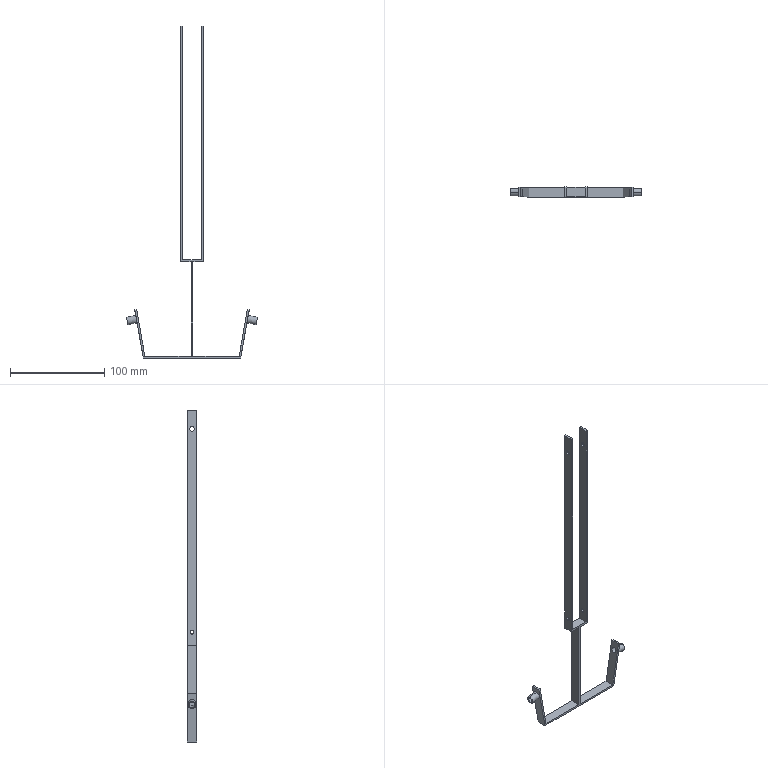Part | SolidWorks | features ICE 6, Extrusion 1, MirrorPattern 1 | 1 solid | 40 faces | box 138.916 x 10 x 352 mm | volume 16665 mm3 | plane 24 | cylinder 16 | commonest cylinder face diameters 4 x4 5 x4 6 x4 8 x4
STEP:
#1=CARTESIAN_POINT('',(12.,5.,10.339));
#2=VERTEX_POINT('',#1);
#3=CARTESIAN_POINT('',(12.,5.,14.339));
#4=VERTEX_POINT('',#3);
#5=CARTESIAN_POINT('',(12.,5.,12.339));
#6=DIRECTION('',(-1.,0.,0.));
#7=DIRECTION('',(0.,0.,1.));
#8=AXIS2_PLACEMENT_3D('',#5,#6,#7);
#9=CIRCLE('',#8,2.);
#10=EDGE_CURVE('',#2,#4,#9,.T.);
#11=ORIENTED_EDGE('',*,*,#10,.F.);
#12=CARTESIAN_POINT('',(10.,5.,10.339));
#13=VERTEX_POINT('',#12);
#14=CARTESIAN_POINT('',(33.,5.,10.339));
#15=DIRECTION('',(-1.,0.,0.));
#16=VECTOR('',#15,1000.);
#17=LINE('',#14,#16);
#18=EDGE_CURVE('',#2,#13,#17,.T.);
#19=ORIENTED_EDGE('',*,*,#18,.T.);
#20=CARTESIAN_POINT('',(10.,5.,14.339));
#21=VERTEX_POINT('',#20);
#22=CARTESIAN_POINT('',(10.,5.,12.339));
#23=DIRECTION('',(1.,0.,0.));
#24=DIRECTION('',(0.,0.,-1.));
#25=AXIS2_PLACEMENT_3D('',#22,#23,#24);
#26=CIRCLE('',#25,2.);
#27=EDGE_CURVE('',#21,#13,#26,.T.);
#28=ORIENTED_EDGE('',*,*,#27,.F.);
#29=CARTESIAN_POINT('',(33.,5.,14.339));
#30=DIRECTION('',(-1.,0.,0.));
#31=VECTOR('',#30,1000.);
#32=LINE('',#29,#31);
#33=EDGE_CURVE('',#4,#21,#32,.T.);
#34=ORIENTED_EDGE('',*,*,#33,.F.);
#35=EDGE_LOOP('',(#11,#19,#28,#34));
#36=FACE_OUTER_BOUND('',#35,.T.);
#37=CARTESIAN_POINT('',(33.,5.,12.339));
#38=DIRECTION('',(-1.,0.,0.));
#39=DIRECTION('',(0.,0.,1.));
#40=AXIS2_PLACEMENT_3D('',#37,#38,#39);
#41=CYLINDRICAL_SURFACE('',#40,2.);
#42=ADVANCED_FACE('',(#36),#41,.F.);
#43=CARTESIAN_POINT('',(-10.,5.,10.339));
#44=VERTEX_POINT('',#43);
#45=CARTESIAN_POINT('',(-10.,5.,14.339));
#46=VERTEX_POINT('',#45);
#47=CARTESIAN_POINT('',(-10.,5.,12.339));
#48=DIRECTION('',(-1.,0.,0.));
#49=DIRECTION('',(0.,0.,1.));
#50=AXIS2_PLACEMENT_3D('',#47,#48,#49);
#51=CIRCLE('',#50,2.);
#52=EDGE_CURVE('',#44,#46,#51,.T.);
#53=ORIENTED_EDGE('',*,*,#52,.F.);
#54=CARTESIAN_POINT('',(-12.,5.,10.339));
#55=VERTEX_POINT('',#54);
#56=CARTESIAN_POINT('',(33.,5.,10.339));
#57=DIRECTION('',(-1.,0.,0.));
#58=VECTOR('',#57,1000.);
#59=LINE('',#56,#58);
#60=EDGE_CURVE('',#44,#55,#59,.T.);
#61=ORIENTED_EDGE('',*,*,#60,.T.);
#62=CARTESIAN_POINT('',(-12.,5.,14.339));
#63=VERTEX_POINT('',#62);
#64=CARTESIAN_POINT('',(-12.,5.,12.339));
#65=DIRECTION('',(-1.,0.,0.));
#66=DIRECTION('',(0.,0.,1.));
#67=AXIS2_PLACEMENT_3D('',#64,#65,#66);
#68=CIRCLE('',#67,2.);
#69=EDGE_CURVE('',#55,#63,#68,.T.);
#70=ORIENTED_EDGE('',*,*,#69,.T.);
#71=CARTESIAN_POINT('',(33.,5.,14.339));
#72=DIRECTION('',(-1.,0.,0.));
#73=VECTOR('',#72,1000.);
#74=LINE('',#71,#73);
#75=EDGE_CURVE('',#46,#63,#74,.T.);
#76=ORIENTED_EDGE('',*,*,#75,.F.);
#77=EDGE_LOOP('',(#53,#61,#70,#76));
#78=FACE_OUTER_BOUND('',#77,.T.);
#79=CARTESIAN_POINT('',(33.,5.,12.339));
#80=DIRECTION('',(-1.,0.,0.));
#81=DIRECTION('',(0.,0.,1.));
#82=AXIS2_PLACEMENT_3D('',#79,#80,#81);
#83=CYLINDRICAL_SURFACE('',#82,2.);
#84=ADVANCED_FACE('',(#78),#83,.F.);
#85=CARTESIAN_POINT('',(12.,5.,225.5));
#86=VERTEX_POINT('',#85);
#87=CARTESIAN_POINT('',(12.,5.,230.5));
#88=VERTEX_POINT('',#87);
#89=CARTESIAN_POINT('',(12.,5.,228.));
#90=DIRECTION('',(-1.,0.,0.));
#91=DIRECTION('',(0.,0.,1.));
#92=AXIS2_PLACEMENT_3D('',#89,#90,#91);
#93=CIRCLE('',#92,2.5);
#94=EDGE_CURVE('',#86,#88,#93,.T.);
#95=ORIENTED_EDGE('',*,*,#94,.F.);
#96=CARTESIAN_POINT('',(10.,5.,225.5));
#97=VERTEX_POINT('',#96);
#98=CARTESIAN_POINT('',(262.,5.,225.5));
#99=DIRECTION('',(-1.,0.,0.));
#100=VECTOR('',#99,1000.);
#101=LINE('',#98,#100);
#102=EDGE_CURVE('',#86,#97,#101,.T.);
#103=ORIENTED_EDGE('',*,*,#102,.T.);
#104=CARTESIAN_POINT('',(10.,5.,230.5));
#105=VERTEX_POINT('',#104);
#106=CARTESIAN_POINT('',(10.,5.,228.));
#107=DIRECTION('',(1.,0.,0.));
#108=DIRECTION('',(0.,0.,-1.));
#109=AXIS2_PLACEMENT_3D('',#106,#107,#108);
#110=CIRCLE('',#109,2.5);
#111=EDGE_CURVE('',#105,#97,#110,.T.);
#112=ORIENTED_EDGE('',*,*,#111,.F.);
#113=CARTESIAN_POINT('',(262.,5.,230.5));
#114=DIRECTION('',(-1.,0.,0.));
#115=VECTOR('',#114,1000.);
#116=LINE('',#113,#115);
#117=EDGE_CURVE('',#88,#105,#116,.T.);
#118=ORIENTED_EDGE('',*,*,#117,.F.);
#119=EDGE_LOOP('',(#95,#103,#112,#118));
#120=FACE_OUTER_BOUND('',#119,.T.);
#121=CARTESIAN_POINT('',(262.,5.,228.));
#122=DIRECTION('',(-1.,0.,0.));
#123=DIRECTION('',(0.,0.,1.));
#124=AXIS2_PLACEMENT_3D('',#121,#122,#123);
#125=CYLINDRICAL_SURFACE('',#124,2.5);
#126=ADVANCED_FACE('',(#120),#125,.F.);
#127=CARTESIAN_POINT('',(-10.,5.,225.5));
#128=VERTEX_POINT('',#127);
#129=CARTESIAN_POINT('',(-10.,5.,230.5));
#130=VERTEX_POINT('',#129);
#131=CARTESIAN_POINT('',(-10.,5.,228.));
#132=DIRECTION('',(-1.,0.,0.));
#133=DIRECTION('',(0.,0.,1.));
#134=AXIS2_PLACEMENT_3D('',#131,#132,#133);
#135=CIRCLE('',#134,2.5);
#136=EDGE_CURVE('',#128,#130,#135,.T.);
#137=ORIENTED_EDGE('',*,*,#136,.F.);
#138=CARTESIAN_POINT('',(-12.,5.,225.5));
#139=VERTEX_POINT('',#138);
#140=CARTESIAN_POINT('',(262.,5.,225.5));
#141=DIRECTION('',(-1.,0.,0.));
#142=VECTOR('',#141,1000.);
#143=LINE('',#140,#142);
#144=EDGE_CURVE('',#128,#139,#143,.T.);
#145=ORIENTED_EDGE('',*,*,#144,.T.);
#146=CARTESIAN_POINT('',(-12.,5.,230.5));
#147=VERTEX_POINT('',#146);
#148=CARTESIAN_POINT('',(-12.,5.,228.));
#149=DIRECTION('',(-1.,0.,0.));
#150=DIRECTION('',(0.,0.,1.));
#151=AXIS2_PLACEMENT_3D('',#148,#149,#150);
#152=CIRCLE('',#151,2.5);
#153=EDGE_CURVE('',#139,#147,#152,.T.);
#154=ORIENTED_EDGE('',*,*,#153,.T.);
#155=CARTESIAN_POINT('',(262.,5.,230.5));
#156=DIRECTION('',(-1.,0.,0.));
#157=VECTOR('',#156,1000.);
#158=LINE('',#155,#157);
#159=EDGE_CURVE('',#130,#147,#158,.T.);
#160=ORIENTED_EDGE('',*,*,#159,.F.);
#161=EDGE_LOOP('',(#137,#145,#154,#160));
#162=FACE_OUTER_BOUND('',#161,.T.);
#163=CARTESIAN_POINT('',(262.,5.,228.));
#164=DIRECTION('',(-1.,0.,0.));
#165=DIRECTION('',(0.,0.,1.));
#166=AXIS2_PLACEMENT_3D('',#163,#164,#165);
#167=CYLINDRICAL_SURFACE('',#166,2.5);
#168=ADVANCED_FACE('',(#162),#167,.F.);
#169=CARTESIAN_POINT('',(68.243,5.,-67.646));
#170=VERTEX_POINT('',#169);
#171=CARTESIAN_POINT('',(69.285,5.,-61.737));
#172=VERTEX_POINT('',#171);
#173=CARTESIAN_POINT('',(68.764,5.,-64.691));
#174=DIRECTION('',(-0.9848,0.,0.1736));
#175=DIRECTION('',(0.1736,0.,0.9848));
#176=AXIS2_PLACEMENT_3D('',#173,#174,#175);
#177=CIRCLE('',#176,3.);
#178=EDGE_CURVE('',#170,#172,#177,.T.);
#179=ORIENTED_EDGE('',*,*,#178,.F.);
#180=CARTESIAN_POINT('',(56.425,5.,-65.562));
#181=VERTEX_POINT('',#180);
#182=CARTESIAN_POINT('',(68.243,5.,-67.646));
#183=DIRECTION('',(-0.9848,0.,0.1736));
#184=VECTOR('',#183,1000.);
#185=LINE('',#182,#184);
#186=EDGE_CURVE('',#170,#181,#185,.T.);
#187=ORIENTED_EDGE('',*,*,#186,.T.);
#188=CARTESIAN_POINT('',(57.467,5.,-59.653));
#189=VERTEX_POINT('',#188);
#190=CARTESIAN_POINT('',(56.946,5.,-62.608));
#191=DIRECTION('',(-0.9848,0.,0.1736));
#192=DIRECTION('',(-0.1736,0.,-0.9848));
#193=AXIS2_PLACEMENT_3D('',#190,#191,#192);
#194=CIRCLE('',#193,3.);
#195=EDGE_CURVE('',#181,#189,#194,.T.);
#196=ORIENTED_EDGE('',*,*,#195,.T.);
#197=CARTESIAN_POINT('',(69.285,5.,-61.737));
#198=DIRECTION('',(-0.9848,0.,0.1736));
#199=VECTOR('',#198,1000.);
#200=LINE('',#197,#199);
#201=EDGE_CURVE('',#172,#189,#200,.T.);
#202=ORIENTED_EDGE('',*,*,#201,.F.);
#203=EDGE_LOOP('',(#179,#187,#196,#202));
#204=FACE_OUTER_BOUND('',#203,.T.);
#205=CARTESIAN_POINT('',(68.764,5.,-64.691));
#206=DIRECTION('',(-0.9848,0.,0.1736));
#207=DIRECTION('',(0.1736,0.,0.9848));
#208=AXIS2_PLACEMENT_3D('',#205,#206,#207);
#209=CYLINDRICAL_SURFACE('',#208,3.);
#210=ADVANCED_FACE('',(#204),#209,.F.);
#211=CARTESIAN_POINT('',(69.458,5.,-60.752));
#212=VERTEX_POINT('',#211);
#213=CARTESIAN_POINT('',(68.069,5.,-68.631));
#214=VERTEX_POINT('',#213);
#215=CARTESIAN_POINT('',(68.764,5.,-64.691));
#216=DIRECTION('',(-0.9848,0.,0.1736));
#217=DIRECTION('',(0.1736,0.,0.9848));
#218=AXIS2_PLACEMENT_3D('',#215,#216,#217);
#219=CIRCLE('',#218,4.);
#220=EDGE_CURVE('',#212,#214,#219,.T.);
#221=ORIENTED_EDGE('',*,*,#220,.T.);
#222=CARTESIAN_POINT('',(58.221,5.,-66.894));
#223=VERTEX_POINT('',#222);
#224=CARTESIAN_POINT('',(68.069,5.,-68.631));
#225=DIRECTION('',(-0.9848,0.,0.1736));
#226=VECTOR('',#225,1000.);
#227=LINE('',#224,#226);
#228=EDGE_CURVE('',#214,#223,#227,.T.);
#229=ORIENTED_EDGE('',*,*,#228,.T.);
#230=CARTESIAN_POINT('',(59.61,5.,-59.016));
#231=VERTEX_POINT('',#230);
#232=CARTESIAN_POINT('',(58.916,5.,-62.955));
#233=DIRECTION('',(-0.9848,0.,0.1736));
#234=DIRECTION('',(0.1736,0.,0.9848));
#235=AXIS2_PLACEMENT_3D('',#232,#233,#234);
#236=CIRCLE('',#235,4.);
#237=EDGE_CURVE('',#231,#223,#236,.T.);
#238=ORIENTED_EDGE('',*,*,#237,.F.);
#239=CARTESIAN_POINT('',(69.458,5.,-60.752));
#240=DIRECTION('',(-0.9848,0.,0.1736));
#241=VECTOR('',#240,1000.);
#242=LINE('',#239,#241);
#243=EDGE_CURVE('',#212,#231,#242,.T.);
#244=ORIENTED_EDGE('',*,*,#243,.F.);
#245=EDGE_LOOP('',(#221,#229,#238,#244));
#246=FACE_OUTER_BOUND('',#245,.T.);
#247=CARTESIAN_POINT('',(68.764,5.,-64.691));
#248=DIRECTION('',(-0.9848,0.,0.1736));
#249=DIRECTION('',(0.1736,0.,0.9848));
#250=AXIS2_PLACEMENT_3D('',#247,#248,#249);
#251=CYLINDRICAL_SURFACE('',#250,4.);
#252=ADVANCED_FACE('',(#246),#251,.T.);
#253=CARTESIAN_POINT('',(-68.243,5.,-67.646));
#254=VERTEX_POINT('',#253);
#255=CARTESIAN_POINT('',(-69.285,5.,-61.737));
#256=VERTEX_POINT('',#255);
#257=CARTESIAN_POINT('',(-68.764,5.,-64.691));
#258=DIRECTION('',(-0.9848,0.,-0.1736));
#259=DIRECTION('',(-0.1736,0.,0.9848));
#260=AXIS2_PLACEMENT_3D('',#257,#258,#259);
#261=CIRCLE('',#260,3.);
#262=EDGE_CURVE('',#254,#256,#261,.T.);
#263=ORIENTED_EDGE('',*,*,#262,.T.);
#264=CARTESIAN_POINT('',(-57.467,5.,-59.653));
#265=VERTEX_POINT('',#264);
#266=CARTESIAN_POINT('',(-69.285,5.,-61.737));
#267=DIRECTION('',(0.9848,0.,0.1736));
#268=VECTOR('',#267,1000.);
#269=LINE('',#266,#268);
#270=EDGE_CURVE('',#256,#265,#269,.T.);
#271=ORIENTED_EDGE('',*,*,#270,.T.);
#272=CARTESIAN_POINT('',(-56.425,5.,-65.562));
#273=VERTEX_POINT('',#272);
#274=CARTESIAN_POINT('',(-56.946,5.,-62.608));
#275=DIRECTION('',(-0.9848,0.,-0.1736));
#276=DIRECTION('',(-0.1736,0.,0.9848));
#277=AXIS2_PLACEMENT_3D('',#274,#275,#276);
#278=CIRCLE('',#277,3.);
#279=EDGE_CURVE('',#273,#265,#278,.T.);
#280=ORIENTED_EDGE('',*,*,#279,.F.);
#281=CARTESIAN_POINT('',(-68.243,5.,-67.646));
#282=DIRECTION('',(0.9848,0.,0.1736));
#283=VECTOR('',#282,1000.);
#284=LINE('',#281,#283);
#285=EDGE_CURVE('',#254,#273,#284,.T.);
#286=ORIENTED_EDGE('',*,*,#285,.F.);
#287=EDGE_LOOP('',(#263,#271,#280,#286));
#288=FACE_OUTER_BOUND('',#287,.T.);
#289=CARTESIAN_POINT('',(-68.764,5.,-64.691));
#290=DIRECTION('',(0.9848,0.,0.1736));
#291=DIRECTION('',(0.1736,0.,-0.9848));
#292=AXIS2_PLACEMENT_3D('',#289,#290,#291);
#293=CYLINDRICAL_SURFACE('',#292,3.);
#294=ADVANCED_FACE('',(#288),#293,.F.);
#295=CARTESIAN_POINT('',(-69.458,5.,-60.752));
#296=VERTEX_POINT('',#295);
#297=CARTESIAN_POINT('',(-68.069,5.,-68.631));
#298=VERTEX_POINT('',#297);
#299=CARTESIAN_POINT('',(-68.764,5.,-64.691));
#300=DIRECTION('',(-0.9848,0.,-0.1736));
#301=DIRECTION('',(-0.1736,0.,0.9848));
#302=AXIS2_PLACEMENT_3D('',#299,#300,#301);
#303=CIRCLE('',#302,4.);
#304=EDGE_CURVE('',#296,#298,#303,.T.);
#305=ORIENTED_EDGE('',*,*,#304,.F.);
#306=CARTESIAN_POINT('',(-59.61,5.,-59.016));
#307=VERTEX_POINT('',#306);
#308=CARTESIAN_POINT('',(-69.458,5.,-60.752));
#309=DIRECTION('',(0.9848,0.,0.1736));
#310=VECTOR('',#309,1000.);
#311=LINE('',#308,#310);
#312=EDGE_CURVE('',#296,#307,#311,.T.);
#313=ORIENTED_EDGE('',*,*,#312,.T.);
#314=CARTESIAN_POINT('',(-58.221,5.,-66.894));
#315=VERTEX_POINT('',#314);
#316=CARTESIAN_POINT('',(-58.916,5.,-62.955));
#317=DIRECTION('',(-0.9848,0.,-0.1736));
#318=DIRECTION('',(0.1736,0.,-0.9848));
#319=AXIS2_PLACEMENT_3D('',#316,#317,#318);
#320=CIRCLE('',#319,4.);
#321=EDGE_CURVE('',#307,#315,#320,.T.);
#322=ORIENTED_EDGE('',*,*,#321,.T.);
#323=CARTESIAN_POINT('',(-68.069,5.,-68.631));
#324=DIRECTION('',(0.9848,0.,0.1736));
#325=VECTOR('',#324,1000.);
#326=LINE('',#323,#325);
#327=EDGE_CURVE('',#298,#315,#326,.T.);
#328=ORIENTED_EDGE('',*,*,#327,.F.);
#329=EDGE_LOOP('',(#305,#313,#322,#328));
#330=FACE_OUTER_BOUND('',#329,.T.);
#331=CARTESIAN_POINT('',(-68.764,5.,-64.691));
#332=DIRECTION('',(0.9848,0.,0.1736));
#333=DIRECTION('',(0.1736,0.,-0.9848));
#334=AXIS2_PLACEMENT_3D('',#331,#332,#333);
#335=CYLINDRICAL_SURFACE('',#334,4.);
#336=ADVANCED_FACE('',(#330),#335,.T.);
#337=CARTESIAN_POINT('',(1.,10.,-2.));
#338=VERTEX_POINT('',#337);
#339=CARTESIAN_POINT('',(1.,0.,-2.));
#340=VERTEX_POINT('',#339);
#341=CARTESIAN_POINT('',(1.,0.,-2.));
#342=DIRECTION('',(0.,-1.,0.));
#343=VECTOR('',#342,1000.);
#344=LINE('',#341,#343);
#345=EDGE_CURVE('',#338,#340,#344,.T.);
#346=ORIENTED_EDGE('',*,*,#345,.F.);
#347=CARTESIAN_POINT('',(12.,10.,-2.));
#348=VERTEX_POINT('',#347);
#349=CARTESIAN_POINT('',(-12.,10.,-2.));
#350=DIRECTION('',(-1.,0.,0.));
#351=VECTOR('',#350,1000.);
#352=LINE('',#349,#351);
#353=EDGE_CURVE('',#348,#338,#352,.T.);
#354=ORIENTED_EDGE('',*,*,#353,.F.);
#355=CARTESIAN_POINT('',(12.,0.,-2.));
#356=VERTEX_POINT('',#355);
#357=CARTESIAN_POINT('',(12.,10.,-2.));
#358=DIRECTION('',(0.,-1.,0.));
#359=VECTOR('',#358,1000.);
#360=LINE('',#357,#359);
#361=EDGE_CURVE('',#348,#356,#360,.T.);
#362=ORIENTED_EDGE('',*,*,#361,.T.);
#363=CARTESIAN_POINT('',(-12.,0.,-2.));
#364=DIRECTION('',(-1.,0.,0.));
#365=VECTOR('',#364,1000.);
#366=LINE('',#363,#365);
#367=EDGE_CURVE('',#356,#340,#366,.T.);
#368=ORIENTED_EDGE('',*,*,#367,.T.);
#369=EDGE_LOOP('',(#346,#354,#362,#368));
#370=FACE_OUTER_BOUND('',#369,.T.);
#371=CARTESIAN_POINT('',(-12.,10.,-2.));
#372=DIRECTION('',(0.,0.,1.));
#373=DIRECTION('',(1.,0.,0.));
#374=AXIS2_PLACEMENT_3D('',#371,#372,#373);
#375=PLANE('',#374);
#376=ADVANCED_FACE('',(#370),#375,.F.);
#377=CARTESIAN_POINT('',(-12.,0.,248.));
#378=VERTEX_POINT('',#377);
#379=CARTESIAN_POINT('',(-10.,0.,248.));
#380=VERTEX_POINT('',#379);
#381=CARTESIAN_POINT('',(-12.,0.,248.));
#382=DIRECTION('',(1.,0.,0.));
#383=VECTOR('',#382,1000.);
#384=LINE('',#381,#383);
#385=EDGE_CURVE('',#378,#380,#384,.T.);
#386=ORIENTED_EDGE('',*,*,#385,.T.);
#387=CARTESIAN_POINT('',(-10.,10.,248.));
#388=VERTEX_POINT('',#387);
#389=CARTESIAN_POINT('',(-10.,10.,248.));
#390=DIRECTION('',(0.,-1.,0.));
#391=VECTOR('',#390,1000.);
#392=LINE('',#389,#391);
#393=EDGE_CURVE('',#388,#380,#392,.T.);
#394=ORIENTED_EDGE('',*,*,#393,.F.);
#395=CARTESIAN_POINT('',(-12.,10.,248.));
#396=VERTEX_POINT('',#395);
#397=CARTESIAN_POINT('',(-12.,10.,248.));
#398=DIRECTION('',(1.,0.,0.));
#399=VECTOR('',#398,1000.);
#400=LINE('',#397,#399);
#401=EDGE_CURVE('',#396,#388,#400,.T.);
#402=ORIENTED_EDGE('',*,*,#401,.F.);
#403=CARTESIAN_POINT('',(-12.,10.,248.));
#404=DIRECTION('',(0.,-1.,0.));
#405=VECTOR('',#404,1000.);
#406=LINE('',#403,#405);
#407=EDGE_CURVE('',#396,#378,#406,.T.);
#408=ORIENTED_EDGE('',*,*,#407,.T.);
#409=EDGE_LOOP('',(#386,#394,#402,#408));
#410=FACE_OUTER_BOUND('',#409,.T.);
#411=CARTESIAN_POINT('',(-12.,10.,248.));
#412=DIRECTION('',(0.,0.,-1.));
#413=DIRECTION('',(-1.,0.,0.));
#414=AXIS2_PLACEMENT_3D('',#411,#412,#413);
#415=PLANE('',#414);
#416=ADVANCED_FACE('',(#410),#415,.F.);
#417=CARTESIAN_POINT('',(-10.,5.,12.339));
#418=DIRECTION('',(-1.,0.,0.));
#419=DIRECTION('',(0.,0.,1.));
#420=AXIS2_PLACEMENT_3D('',#417,#418,#419);
#421=CIRCLE('',#420,2.);
#422=EDGE_CURVE('',#46,#44,#421,.T.);
#423=ORIENTED_EDGE('',*,*,#422,.T.);
#424=ORIENTED_EDGE('',*,*,#52,.T.);
#425=EDGE_LOOP('',(#423,#424));
#426=FACE_BOUND('',#425,.T.);
#427=CARTESIAN_POINT('',(-10.,5.,228.));
#428=DIRECTION('',(-1.,0.,0.));
#429=DIRECTION('',(0.,0.,1.));
#430=AXIS2_PLACEMENT_3D('',#427,#428,#429);
#431=CIRCLE('',#430,2.5);
#432=EDGE_CURVE('',#130,#128,#431,.T.);
#433=ORIENTED_EDGE('',*,*,#432,.T.);
#434=ORIENTED_EDGE('',*,*,#136,.T.);
#435=EDGE_LOOP('',(#433,#434));
#436=FACE_BOUND('',#435,.T.);
#437=CARTESIAN_POINT('',(-10.,0.,0.));
#438=VERTEX_POINT('',#437);
#439=CARTESIAN_POINT('',(-10.,0.,248.));
#440=DIRECTION('',(0.,0.,-1.));
#441=VECTOR('',#440,1000.);
#442=LINE('',#439,#441);
#443=EDGE_CURVE('',#380,#438,#442,.T.);
#444=ORIENTED_EDGE('',*,*,#443,.T.);
#445=CARTESIAN_POINT('',(-10.,10.,0.));
#446=VERTEX_POINT('',#445);
#447=CARTESIAN_POINT('',(-10.,10.,0.));
#448=DIRECTION('',(0.,-1.,0.));
#449=VECTOR('',#448,1000.);
#450=LINE('',#447,#449);
#451=EDGE_CURVE('',#446,#438,#450,.T.);
#452=ORIENTED_EDGE('',*,*,#451,.F.);
#453=CARTESIAN_POINT('',(-10.,10.,248.));
#454=DIRECTION('',(0.,0.,-1.));
#455=VECTOR('',#454,1000.);
#456=LINE('',#453,#455);
#457=EDGE_CURVE('',#388,#446,#456,.T.);
#458=ORIENTED_EDGE('',*,*,#457,.F.);
#459=ORIENTED_EDGE('',*,*,#393,.T.);
#460=EDGE_LOOP('',(#444,#452,#458,#459));
#461=FACE_OUTER_BOUND('',#460,.T.);
#462=CARTESIAN_POINT('',(-10.,10.,248.));
#463=DIRECTION('',(-1.,0.,0.));
#464=DIRECTION('',(0.,0.,1.));
#465=AXIS2_PLACEMENT_3D('',#462,#463,#464);
#466=PLANE('',#465);
#467=ADVANCED_FACE('',(#426,#436,#461),#466,.F.);
#468=CARTESIAN_POINT('',(10.,0.,0.));
#469=VERTEX_POINT('',#468);
#470=CARTESIAN_POINT('',(-10.,0.,0.));
#471=DIRECTION('',(1.,0.,0.));
#472=VECTOR('',#471,1000.);
#473=LINE('',#470,#472);
#474=EDGE_CURVE('',#438,#469,#473,.T.);
#475=ORIENTED_EDGE('',*,*,#474,.T.);
#476=CARTESIAN_POINT('',(10.,10.,0.));
#477=VERTEX_POINT('',#476);
#478=CARTESIAN_POINT('',(10.,10.,0.));
#479=DIRECTION('',(0.,-1.,0.));
#480=VECTOR('',#479,1000.);
#481=LINE('',#478,#480);
#482=EDGE_CURVE('',#477,#469,#481,.T.);
#483=ORIENTED_EDGE('',*,*,#482,.F.);
#484=CARTESIAN_POINT('',(-10.,10.,0.));
#485=DIRECTION('',(1.,0.,0.));
#486=VECTOR('',#485,1000.);
#487=LINE('',#484,#486);
#488=EDGE_CURVE('',#446,#477,#487,.T.);
#489=ORIENTED_EDGE('',*,*,#488,.F.);
#490=ORIENTED_EDGE('',*,*,#451,.T.);
#491=EDGE_LOOP('',(#475,#483,#489,#490));
#492=FACE_OUTER_BOUND('',#491,.T.);
#493=CARTESIAN_POINT('',(-10.,10.,0.));
#494=DIRECTION('',(0.,0.,-1.));
#495=DIRECTION('',(-1.,0.,0.));
#496=AXIS2_PLACEMENT_3D('',#493,#494,#495);
#497=PLANE('',#496);
#498=ADVANCED_FACE('',(#492),#497,.F.);
#499=ORIENTED_EDGE('',*,*,#27,.T.);
#500=CARTESIAN_POINT('',(10.,5.,12.339));
#501=DIRECTION('',(1.,0.,0.));
#502=DIRECTION('',(0.,0.,-1.));
#503=AXIS2_PLACEMENT_3D('',#500,#501,#502);
#504=CIRCLE('',#503,2.);
#505=EDGE_CURVE('',#13,#21,#504,.T.);
#506=ORIENTED_EDGE('',*,*,#505,.T.);
#507=EDGE_LOOP('',(#499,#506));
#508=FACE_BOUND('',#507,.T.);
#509=ORIENTED_EDGE('',*,*,#111,.T.);
#510=CARTESIAN_POINT('',(10.,5.,228.));
#511=DIRECTION('',(1.,0.,0.));
#512=DIRECTION('',(0.,0.,-1.));
#513=AXIS2_PLACEMENT_3D('',#510,#511,#512);
#514=CIRCLE('',#513,2.5);
#515=EDGE_CURVE('',#97,#105,#514,.T.);
#516=ORIENTED_EDGE('',*,*,#515,.T.);
#517=EDGE_LOOP('',(#509,#516));
#518=FACE_BOUND('',#517,.T.);
#519=CARTESIAN_POINT('',(10.,0.,248.));
#520=VERTEX_POINT('',#519);
#521=CARTESIAN_POINT('',(10.,0.,0.));
#522=DIRECTION('',(0.,0.,1.));
#523=VECTOR('',#522,1000.);
#524=LINE('',#521,#523);
#525=EDGE_CURVE('',#469,#520,#524,.T.);
#526=ORIENTED_EDGE('',*,*,#525,.T.);
#527=CARTESIAN_POINT('',(10.,10.,248.));
#528=VERTEX_POINT('',#527);
#529=CARTESIAN_POINT('',(10.,10.,248.));
#530=DIRECTION('',(0.,-1.,0.));
#531=VECTOR('',#530,1000.);
#532=LINE('',#529,#531);
#533=EDGE_CURVE('',#528,#520,#532,.T.);
#534=ORIENTED_EDGE('',*,*,#533,.F.);
#535=CARTESIAN_POINT('',(10.,10.,0.));
#536=DIRECTION('',(0.,0.,1.));
#537=VECTOR('',#536,1000.);
#538=LINE('',#535,#537);
#539=EDGE_CURVE('',#477,#528,#538,.T.);
#540=ORIENTED_EDGE('',*,*,#539,.F.);
#541=ORIENTED_EDGE('',*,*,#482,.T.);
#542=EDGE_LOOP('',(#526,#534,#540,#541));
#543=FACE_OUTER_BOUND('',#542,.T.);
#544=CARTESIAN_POINT('',(10.,10.,0.));
#545=DIRECTION('',(1.,0.,0.));
#546=DIRECTION('',(0.,0.,-1.));
#547=AXIS2_PLACEMENT_3D('',#544,#545,#546);
#548=PLANE('',#547);
#549=ADVANCED_FACE('',(#508,#518,#543),#548,.F.);
#550=CARTESIAN_POINT('',(12.,0.,248.));
#551=VERTEX_POINT('',#550);
#552=CARTESIAN_POINT('',(10.,0.,248.));
#553=DIRECTION('',(1.,0.,0.));
#554=VECTOR('',#553,1000.);
#555=LINE('',#552,#554);
#556=EDGE_CURVE('',#520,#551,#555,.T.);
#557=ORIENTED_EDGE('',*,*,#556,.T.);
#558=CARTESIAN_POINT('',(12.,10.,248.));
#559=VERTEX_POINT('',#558);
#560=CARTESIAN_POINT('',(12.,10.,248.));
#561=DIRECTION('',(0.,-1.,0.));
#562=VECTOR('',#561,1000.);
#563=LINE('',#560,#562);
#564=EDGE_CURVE('',#559,#551,#563,.T.);
#565=ORIENTED_EDGE('',*,*,#564,.F.);
#566=CARTESIAN_POINT('',(10.,10.,248.));
#567=DIRECTION('',(1.,0.,0.));
#568=VECTOR('',#567,1000.);
#569=LINE('',#566,#568);
#570=EDGE_CURVE('',#528,#559,#569,.T.);
#571=ORIENTED_EDGE('',*,*,#570,.F.);
#572=ORIENTED_EDGE('',*,*,#533,.T.);
#573=EDGE_LOOP('',(#557,#565,#571,#572));
#574=FACE_OUTER_BOUND('',#573,.T.);
#575=CARTESIAN_POINT('',(10.,10.,248.));
#576=DIRECTION('',(0.,0.,-1.));
#577=DIRECTION('',(-1.,0.,0.));
#578=AXIS2_PLACEMENT_3D('',#575,#576,#577);
#579=PLANE('',#578);
#580=ADVANCED_FACE('',(#574),#579,.F.);
#581=CARTESIAN_POINT('',(12.,5.,12.339));
#582=DIRECTION('',(-1.,0.,0.));
#583=DIRECTION('',(0.,0.,1.));
#584=AXIS2_PLACEMENT_3D('',#581,#582,#583);
#585=CIRCLE('',#584,2.);
#586=EDGE_CURVE('',#4,#2,#585,.T.);
#587=ORIENTED_EDGE('',*,*,#586,.T.);
#588=ORIENTED_EDGE('',*,*,#10,.T.);
#589=EDGE_LOOP('',(#587,#588));
#590=FACE_BOUND('',#589,.T.);
#591=CARTESIAN_POINT('',(12.,5.,228.));
#592=DIRECTION('',(-1.,0.,0.));
#593=DIRECTION('',(0.,0.,1.));
#594=AXIS2_PLACEMENT_3D('',#591,#592,#593);
#595=CIRCLE('',#594,2.5);
#596=EDGE_CURVE('',#88,#86,#595,.T.);
#597=ORIENTED_EDGE('',*,*,#596,.T.);
#598=ORIENTED_EDGE('',*,*,#94,.T.);
#599=EDGE_LOOP('',(#597,#598));
#600=FACE_BOUND('',#599,.T.);
#601=CARTESIAN_POINT('',(12.,0.,-2.));
#602=DIRECTION('',(0.,0.,-1.));
#603=VECTOR('',#602,1000.);
#604=LINE('',#601,#603);
#605=EDGE_CURVE('',#551,#356,#604,.T.);
#606=ORIENTED_EDGE('',*,*,#605,.T.);
#607=ORIENTED_EDGE('',*,*,#361,.F.);
#608=CARTESIAN_POINT('',(12.,10.,-2.));
#609=DIRECTION('',(0.,0.,-1.));
#610=VECTOR('',#609,1000.);
#611=LINE('',#608,#610);
#612=EDGE_CURVE('',#559,#348,#611,.T.);
#613=ORIENTED_EDGE('',*,*,#612,.F.);
#614=ORIENTED_EDGE('',*,*,#564,.T.);
#615=EDGE_LOOP('',(#606,#607,#613,#614));
#616=FACE_OUTER_BOUND('',#615,.T.);
#617=CARTESIAN_POINT('',(12.,10.,-2.));
#618=DIRECTION('',(-1.,0.,0.));
#619=DIRECTION('',(0.,0.,1.));
#620=AXIS2_PLACEMENT_3D('',#617,#618,#619);
#621=PLANE('',#620);
#622=ADVANCED_FACE('',(#590,#600,#616),#621,.F.);
#623=CARTESIAN_POINT('',(-1.,10.,-2.));
#624=VERTEX_POINT('',#623);
#625=CARTESIAN_POINT('',(-12.,10.,-2.));
#626=VERTEX_POINT('',#625);
#627=CARTESIAN_POINT('',(-12.,10.,-2.));
#628=DIRECTION('',(-1.,0.,0.));
#629=VECTOR('',#628,1000.);
#630=LINE('',#627,#629);
#631=EDGE_CURVE('',#624,#626,#630,.T.);
#632=ORIENTED_EDGE('',*,*,#631,.F.);
#633=CARTESIAN_POINT('',(-1.,0.,-2.));
#634=VERTEX_POINT('',#633);
#635=CARTESIAN_POINT('',(-1.,0.,-2.));
#636=DIRECTION('',(0.,-1.,0.));
#637=VECTOR('',#636,1000.);
#638=LINE('',#635,#637);
#639=EDGE_CURVE('',#624,#634,#638,.T.);
#640=ORIENTED_EDGE('',*,*,#639,.T.);
#641=CARTESIAN_POINT('',(-12.,0.,-2.));
#642=VERTEX_POINT('',#641);
#643=CARTESIAN_POINT('',(-12.,0.,-2.));
#644=DIRECTION('',(-1.,0.,0.));
#645=VECTOR('',#644,1000.);
#646=LINE('',#643,#645);
#647=EDGE_CURVE('',#634,#642,#646,.T.);
#648=ORIENTED_EDGE('',*,*,#647,.T.);
#649=CARTESIAN_POINT('',(-12.,10.,-2.));
#650=DIRECTION('',(0.,-1.,0.));
#651=VECTOR('',#650,1000.);
#652=LINE('',#649,#651);
#653=EDGE_CURVE('',#626,#642,#652,.T.);
#654=ORIENTED_EDGE('',*,*,#653,.F.);
#655=EDGE_LOOP('',(#632,#640,#648,#654));
#656=FACE_OUTER_BOUND('',#655,.T.);
#657=CARTESIAN_POINT('',(-12.,10.,-2.));
#658=DIRECTION('',(0.,0.,1.));
#659=DIRECTION('',(1.,0.,0.));
#660=AXIS2_PLACEMENT_3D('',#657,#658,#659);
#661=PLANE('',#660);
#662=ADVANCED_FACE('',(#656),#661,.F.);
#663=CARTESIAN_POINT('',(-12.,5.,12.339));
#664=DIRECTION('',(-1.,0.,0.));
#665=DIRECTION('',(0.,0.,1.));
#666=AXIS2_PLACEMENT_3D('',#663,#664,#665);
#667=CIRCLE('',#666,2.);
#668=EDGE_CURVE('',#63,#55,#667,.T.);
#669=ORIENTED_EDGE('',*,*,#668,.F.);
#670=ORIENTED_EDGE('',*,*,#69,.F.);
#671=EDGE_LOOP('',(#669,#670));
#672=FACE_BOUND('',#671,.T.);
#673=CARTESIAN_POINT('',(-12.,5.,228.));
#674=DIRECTION('',(-1.,0.,0.));
#675=DIRECTION('',(0.,0.,1.));
#676=AXIS2_PLACEMENT_3D('',#673,#674,#675);
#677=CIRCLE('',#676,2.5);
#678=EDGE_CURVE('',#147,#139,#677,.T.);
#679=ORIENTED_EDGE('',*,*,#678,.F.);
#680=ORIENTED_EDGE('',*,*,#153,.F.);
#681=EDGE_LOOP('',(#679,#680));
#682=FACE_BOUND('',#681,.T.);
#683=CARTESIAN_POINT('',(-12.,0.,248.));
#684=DIRECTION('',(0.,0.,1.));
#685=VECTOR('',#684,1000.);
#686=LINE('',#683,#685);
#687=EDGE_CURVE('',#642,#378,#686,.T.);
#688=ORIENTED_EDGE('',*,*,#687,.T.);
#689=ORIENTED_EDGE('',*,*,#407,.F.);
#690=CARTESIAN_POINT('',(-12.,10.,248.));
#691=DIRECTION('',(0.,0.,1.));
#692=VECTOR('',#691,1000.);
#693=LINE('',#690,#692);
#694=EDGE_CURVE('',#626,#396,#693,.T.);
#695=ORIENTED_EDGE('',*,*,#694,.F.);
#696=ORIENTED_EDGE('',*,*,#653,.T.);
#697=EDGE_LOOP('',(#688,#689,#695,#696));
#698=FACE_OUTER_BOUND('',#697,.T.);
#699=CARTESIAN_POINT('',(-12.,10.,248.));
#700=DIRECTION('',(1.,0.,0.));
#701=DIRECTION('',(0.,0.,-1.));
#702=AXIS2_PLACEMENT_3D('',#699,#700,#701);
#703=PLANE('',#702);
#704=ADVANCED_FACE('',(#672,#682,#698),#703,.F.);
#705=ORIENTED_EDGE('',*,*,#401,.T.);
#706=ORIENTED_EDGE('',*,*,#457,.T.);
#707=ORIENTED_EDGE('',*,*,#488,.T.);
#708=ORIENTED_EDGE('',*,*,#539,.T.);
#709=ORIENTED_EDGE('',*,*,#570,.T.);
#710=ORIENTED_EDGE('',*,*,#612,.T.);
#711=ORIENTED_EDGE('',*,*,#353,.T.);
#712=CARTESIAN_POINT('',(1.,10.,-102.));
#713=VERTEX_POINT('',#712);
#714=CARTESIAN_POINT('',(1.,10.,-2.));
#715=DIRECTION('',(0.,0.,1.));
#716=VECTOR('',#715,1000.);
#717=LINE('',#714,#716);
#718=EDGE_CURVE('',#713,#338,#717,.T.);
#719=ORIENTED_EDGE('',*,*,#718,.F.);
#720=CARTESIAN_POINT('',(50.,10.,-102.));
#721=VERTEX_POINT('',#720);
#722=CARTESIAN_POINT('',(-50.,10.,-102.));
#723=DIRECTION('',(1.,0.,0.));
#724=VECTOR('',#723,1000.);
#725=LINE('',#722,#724);
#726=EDGE_CURVE('',#713,#721,#725,.T.);
#727=ORIENTED_EDGE('',*,*,#726,.T.);
#728=CARTESIAN_POINT('',(58.682,10.,-52.76));
#729=VERTEX_POINT('',#728);
#730=CARTESIAN_POINT('',(50.,10.,-102.));
#731=DIRECTION('',(0.1736,0.,0.9848));
#732=VECTOR('',#731,1000.);
#733=LINE('',#730,#732);
#734=EDGE_CURVE('',#721,#729,#733,.T.);
#735=ORIENTED_EDGE('',*,*,#734,.T.);
#736=CARTESIAN_POINT('',(60.652,10.,-53.107));
#737=VERTEX_POINT('',#736);
#738=CARTESIAN_POINT('',(60.652,10.,-53.107));
#739=DIRECTION('',(0.9848,0.,-0.1736));
#740=VECTOR('',#739,1000.);
#741=LINE('',#738,#740);
#742=EDGE_CURVE('',#729,#737,#741,.T.);
#743=ORIENTED_EDGE('',*,*,#742,.T.);
#744=CARTESIAN_POINT('',(51.678,10.,-104.));
#745=VERTEX_POINT('',#744);
#746=CARTESIAN_POINT('',(51.678,10.,-104.));
#747=DIRECTION('',(-0.1736,0.,-0.9848));
#748=VECTOR('',#747,1000.);
#749=LINE('',#746,#748);
#750=EDGE_CURVE('',#737,#745,#749,.T.);
#751=ORIENTED_EDGE('',*,*,#750,.T.);
#752=CARTESIAN_POINT('',(-51.678,10.,-104.));
#753=VERTEX_POINT('',#752);
#754=CARTESIAN_POINT('',(-51.678,10.,-104.));
#755=DIRECTION('',(-1.,0.,0.));
#756=VECTOR('',#755,1000.);
#757=LINE('',#754,#756);
#758=EDGE_CURVE('',#745,#753,#757,.T.);
#759=ORIENTED_EDGE('',*,*,#758,.T.);
#760=CARTESIAN_POINT('',(-60.652,10.,-53.107));
#761=VERTEX_POINT('',#760);
#762=CARTESIAN_POINT('',(-51.678,10.,-104.));
#763=DIRECTION('',(-0.1736,0.,0.9848));
#764=VECTOR('',#763,1000.);
#765=LINE('',#762,#764);
#766=EDGE_CURVE('',#753,#761,#765,.T.);
#767=ORIENTED_EDGE('',*,*,#766,.T.);
#768=CARTESIAN_POINT('',(-58.682,10.,-52.76));
#769=VERTEX_POINT('',#768);
#770=CARTESIAN_POINT('',(-58.682,10.,-52.76));
#771=DIRECTION('',(0.9848,0.,0.1736));
#772=VECTOR('',#771,1000.);
#773=LINE('',#770,#772);
#774=EDGE_CURVE('',#761,#769,#773,.T.);
#775=ORIENTED_EDGE('',*,*,#774,.T.);
#776=CARTESIAN_POINT('',(-50.,10.,-102.));
#777=VERTEX_POINT('',#776);
#778=CARTESIAN_POINT('',(-50.,10.,-102.));
#779=DIRECTION('',(0.1736,0.,-0.9848));
#780=VECTOR('',#779,1000.);
#781=LINE('',#778,#780);
#782=EDGE_CURVE('',#769,#777,#781,.T.);
#783=ORIENTED_EDGE('',*,*,#782,.T.);
#784=CARTESIAN_POINT('',(-1.,10.,-102.));
#785=VERTEX_POINT('',#784);
#786=CARTESIAN_POINT('',(-50.,10.,-102.));
#787=DIRECTION('',(1.,0.,0.));
#788=VECTOR('',#787,1000.);
#789=LINE('',#786,#788);
#790=EDGE_CURVE('',#777,#785,#789,.T.);
#791=ORIENTED_EDGE('',*,*,#790,.T.);
#792=CARTESIAN_POINT('',(-1.,10.,-2.));
#793=DIRECTION('',(0.,0.,1.));
#794=VECTOR('',#793,1000.);
#795=LINE('',#792,#794);
#796=EDGE_CURVE('',#785,#624,#795,.T.);
#797=ORIENTED_EDGE('',*,*,#796,.T.);
#798=ORIENTED_EDGE('',*,*,#631,.T.);
#799=ORIENTED_EDGE('',*,*,#694,.T.);
#800=EDGE_LOOP('',(#705,#706,#707,#708,#709,#710,#711,#719,#727,#735,#743,#751,#759,#767,#775,#783,#791,#797,#798,#799));
#801=FACE_OUTER_BOUND('',#800,.T.);
#802=CARTESIAN_POINT('',(0.,10.,0.));
#803=DIRECTION('',(0.,1.,0.));
#804=DIRECTION('',(0.,0.,1.));
#805=AXIS2_PLACEMENT_3D('',#802,#803,#804);
#806=PLANE('',#805);
#807=ADVANCED_FACE('',(#801),#806,.T.);
#808=ORIENTED_EDGE('',*,*,#385,.F.);
#809=ORIENTED_EDGE('',*,*,#687,.F.);
#810=ORIENTED_EDGE('',*,*,#647,.F.);
#811=CARTESIAN_POINT('',(-1.,0.,-102.));
#812=VERTEX_POINT('',#811);
#813=CARTESIAN_POINT('',(-1.,0.,-102.));
#814=DIRECTION('',(0.,0.,-1.));
#815=VECTOR('',#814,1000.);
#816=LINE('',#813,#815);
#817=EDGE_CURVE('',#634,#812,#816,.T.);
#818=ORIENTED_EDGE('',*,*,#817,.T.);
#819=CARTESIAN_POINT('',(-50.,0.,-102.));
#820=VERTEX_POINT('',#819);
#821=CARTESIAN_POINT('',(-50.,0.,-102.));
#822=DIRECTION('',(1.,0.,0.));
#823=VECTOR('',#822,1000.);
#824=LINE('',#821,#823);
#825=EDGE_CURVE('',#820,#812,#824,.T.);
#826=ORIENTED_EDGE('',*,*,#825,.F.);
#827=CARTESIAN_POINT('',(-58.682,0.,-52.76));
#828=VERTEX_POINT('',#827);
#829=CARTESIAN_POINT('',(-50.,0.,-102.));
#830=DIRECTION('',(0.1736,0.,-0.9848));
#831=VECTOR('',#830,1000.);
#832=LINE('',#829,#831);
#833=EDGE_CURVE('',#828,#820,#832,.T.);
#834=ORIENTED_EDGE('',*,*,#833,.F.);
#835=CARTESIAN_POINT('',(-60.652,0.,-53.107));
#836=VERTEX_POINT('',#835);
#837=CARTESIAN_POINT('',(-58.682,0.,-52.76));
#838=DIRECTION('',(0.9848,0.,0.1736));
#839=VECTOR('',#838,1000.);
#840=LINE('',#837,#839);
#841=EDGE_CURVE('',#836,#828,#840,.T.);
#842=ORIENTED_EDGE('',*,*,#841,.F.);
#843=CARTESIAN_POINT('',(-51.678,0.,-104.));
#844=VERTEX_POINT('',#843);
#845=CARTESIAN_POINT('',(-51.678,0.,-104.));
#846=DIRECTION('',(-0.1736,0.,0.9848));
#847=VECTOR('',#846,1000.);
#848=LINE('',#845,#847);
#849=EDGE_CURVE('',#844,#836,#848,.T.);
#850=ORIENTED_EDGE('',*,*,#849,.F.);
#851=CARTESIAN_POINT('',(51.678,0.,-104.));
#852=VERTEX_POINT('',#851);
#853=CARTESIAN_POINT('',(-51.678,0.,-104.));
#854=DIRECTION('',(-1.,0.,0.));
#855=VECTOR('',#854,1000.);
#856=LINE('',#853,#855);
#857=EDGE_CURVE('',#852,#844,#856,.T.);
#858=ORIENTED_EDGE('',*,*,#857,.F.);
#859=CARTESIAN_POINT('',(60.652,0.,-53.107));
#860=VERTEX_POINT('',#859);
#861=CARTESIAN_POINT('',(51.678,0.,-104.));
#862=DIRECTION('',(-0.1736,0.,-0.9848));
#863=VECTOR('',#862,1000.);
#864=LINE('',#861,#863);
#865=EDGE_CURVE('',#860,#852,#864,.T.);
#866=ORIENTED_EDGE('',*,*,#865,.F.);
#867=CARTESIAN_POINT('',(58.682,0.,-52.76));
#868=VERTEX_POINT('',#867);
#869=CARTESIAN_POINT('',(60.652,0.,-53.107));
#870=DIRECTION('',(0.9848,0.,-0.1736));
#871=VECTOR('',#870,1000.);
#872=LINE('',#869,#871);
#873=EDGE_CURVE('',#868,#860,#872,.T.);
#874=ORIENTED_EDGE('',*,*,#873,.F.);
#875=CARTESIAN_POINT('',(50.,0.,-102.));
#876=VERTEX_POINT('',#875);
#877=CARTESIAN_POINT('',(50.,0.,-102.));
#878=DIRECTION('',(0.1736,0.,0.9848));
#879=VECTOR('',#878,1000.);
#880=LINE('',#877,#879);
#881=EDGE_CURVE('',#876,#868,#880,.T.);
#882=ORIENTED_EDGE('',*,*,#881,.F.);
#883=CARTESIAN_POINT('',(1.,0.,-102.));
#884=VERTEX_POINT('',#883);
#885=CARTESIAN_POINT('',(-50.,0.,-102.));
#886=DIRECTION('',(1.,0.,0.));
#887=VECTOR('',#886,1000.);
#888=LINE('',#885,#887);
#889=EDGE_CURVE('',#884,#876,#888,.T.);
#890=ORIENTED_EDGE('',*,*,#889,.F.);
#891=CARTESIAN_POINT('',(1.,0.,-102.));
#892=DIRECTION('',(0.,0.,-1.));
#893=VECTOR('',#892,1000.);
#894=LINE('',#891,#893);
#895=EDGE_CURVE('',#340,#884,#894,.T.);
#896=ORIENTED_EDGE('',*,*,#895,.F.);
#897=ORIENTED_EDGE('',*,*,#367,.F.);
#898=ORIENTED_EDGE('',*,*,#605,.F.);
#899=ORIENTED_EDGE('',*,*,#556,.F.);
#900=ORIENTED_EDGE('',*,*,#525,.F.);
#901=ORIENTED_EDGE('',*,*,#474,.F.);
#902=ORIENTED_EDGE('',*,*,#443,.F.);
#903=EDGE_LOOP('',(#808,#809,#810,#818,#826,#834,#842,#850,#858,#866,#874,#882,#890,#896,#897,#898,#899,#900,#901,#902));
#904=FACE_OUTER_BOUND('',#903,.T.);
#905=CARTESIAN_POINT('',(0.,0.,0.));
#906=DIRECTION('',(0.,1.,0.));
#907=DIRECTION('',(0.,0.,1.));
#908=AXIS2_PLACEMENT_3D('',#905,#906,#907);
#909=PLANE('',#908);
#910=ADVANCED_FACE('',(#904),#909,.F.);
#911=ORIENTED_EDGE('',*,*,#345,.T.);
#912=ORIENTED_EDGE('',*,*,#895,.T.);
#913=CARTESIAN_POINT('',(1.,10.,-102.));
#914=DIRECTION('',(0.,1.,0.));
#915=VECTOR('',#914,1000.);
#916=LINE('',#913,#915);
#917=EDGE_CURVE('',#884,#713,#916,.T.);
#918=ORIENTED_EDGE('',*,*,#917,.T.);
#919=ORIENTED_EDGE('',*,*,#718,.T.);
#920=EDGE_LOOP('',(#911,#912,#918,#919));
#921=FACE_OUTER_BOUND('',#920,.T.);
#922=CARTESIAN_POINT('',(1.,0.,0.));
#923=DIRECTION('',(-1.,0.,0.));
#924=DIRECTION('',(0.,0.,1.));
#925=AXIS2_PLACEMENT_3D('',#922,#923,#924);
#926=PLANE('',#925);
#927=ADVANCED_FACE('',(#921),#926,.F.);
#928=ORIENTED_EDGE('',*,*,#639,.F.);
#929=ORIENTED_EDGE('',*,*,#796,.F.);
#930=CARTESIAN_POINT('',(-1.,10.,-102.));
#931=DIRECTION('',(0.,1.,0.));
#932=VECTOR('',#931,1000.);
#933=LINE('',#930,#932);
#934=EDGE_CURVE('',#812,#785,#933,.T.);
#935=ORIENTED_EDGE('',*,*,#934,.F.);
#936=ORIENTED_EDGE('',*,*,#817,.F.);
#937=EDGE_LOOP('',(#928,#929,#935,#936));
#938=FACE_OUTER_BOUND('',#937,.T.);
#939=CARTESIAN_POINT('',(-1.,0.,0.));
#940=DIRECTION('',(-1.,0.,0.));
#941=DIRECTION('',(0.,0.,1.));
#942=AXIS2_PLACEMENT_3D('',#939,#940,#941);
#943=PLANE('',#942);
#944=ADVANCED_FACE('',(#938),#943,.T.);
#945=ORIENTED_EDGE('',*,*,#726,.F.);
#946=ORIENTED_EDGE('',*,*,#917,.F.);
#947=ORIENTED_EDGE('',*,*,#889,.T.);
#948=CARTESIAN_POINT('',(50.,10.,-102.));
#949=DIRECTION('',(0.,-1.,0.));
#950=VECTOR('',#949,1000.);
#951=LINE('',#948,#950);
#952=EDGE_CURVE('',#721,#876,#951,.T.);
#953=ORIENTED_EDGE('',*,*,#952,.F.);
#954=EDGE_LOOP('',(#945,#946,#947,#953));
#955=FACE_OUTER_BOUND('',#954,.T.);
#956=CARTESIAN_POINT('',(-50.,10.,-102.));
#957=DIRECTION('',(0.,0.,-1.));
#958=DIRECTION('',(-1.,0.,0.));
#959=AXIS2_PLACEMENT_3D('',#956,#957,#958);
#960=PLANE('',#959);
#961=ADVANCED_FACE('',(#955),#960,.F.);
#962=ORIENTED_EDGE('',*,*,#279,.T.);
#963=CARTESIAN_POINT('',(-56.946,5.,-62.608));
#964=DIRECTION('',(-0.9848,0.,-0.1736));
#965=DIRECTION('',(-0.1736,0.,0.9848));
#966=AXIS2_PLACEMENT_3D('',#963,#964,#965);
#967=CIRCLE('',#966,3.);
#968=EDGE_CURVE('',#265,#273,#967,.T.);
#969=ORIENTED_EDGE('',*,*,#968,.T.);
#970=EDGE_LOOP('',(#962,#969));
#971=FACE_BOUND('',#970,.T.);
#972=ORIENTED_EDGE('',*,*,#833,.T.);
#973=CARTESIAN_POINT('',(-50.,10.,-102.));
#974=DIRECTION('',(0.,-1.,0.));
#975=VECTOR('',#974,1000.);
#976=LINE('',#973,#975);
#977=EDGE_CURVE('',#777,#820,#976,.T.);
#978=ORIENTED_EDGE('',*,*,#977,.F.);
#979=ORIENTED_EDGE('',*,*,#782,.F.);
#980=CARTESIAN_POINT('',(-58.682,10.,-52.76));
#981=DIRECTION('',(0.,-1.,0.));
#982=VECTOR('',#981,1000.);
#983=LINE('',#980,#982);
#984=EDGE_CURVE('',#769,#828,#983,.T.);
#985=ORIENTED_EDGE('',*,*,#984,.T.);
#986=EDGE_LOOP('',(#972,#978,#979,#985));
#987=FACE_OUTER_BOUND('',#986,.T.);
#988=CARTESIAN_POINT('',(-50.,10.,-102.));
#989=DIRECTION('',(-0.9848,0.,-0.1736));
#990=DIRECTION('',(-0.1736,0.,0.9848));
#991=AXIS2_PLACEMENT_3D('',#988,#989,#990);
#992=PLANE('',#991);
#993=ADVANCED_FACE('',(#971,#987),#992,.F.);
#994=ORIENTED_EDGE('',*,*,#934,.T.);
#995=ORIENTED_EDGE('',*,*,#790,.F.);
#996=ORIENTED_EDGE('',*,*,#977,.T.);
#997=ORIENTED_EDGE('',*,*,#825,.T.);
#998=EDGE_LOOP('',(#994,#995,#996,#997));
#999=FACE_OUTER_BOUND('',#998,.T.);
#1000=CARTESIAN_POINT('',(-50.,10.,-102.));
#1001=DIRECTION('',(0.,0.,-1.));
#1002=DIRECTION('',(-1.,0.,0.));
#1003=AXIS2_PLACEMENT_3D('',#1000,#1001,#1002);
#1004=PLANE('',#1003);
#1005=ADVANCED_FACE('',(#999),#1004,.F.);
#1006=CARTESIAN_POINT('',(56.946,5.,-62.608));
#1007=DIRECTION('',(-0.9848,0.,0.1736));
#1008=DIRECTION('',(-0.1736,0.,-0.9848));
#1009=AXIS2_PLACEMENT_3D('',#1006,#1007,#1008);
#1010=CIRCLE('',#1009,3.);
#1011=EDGE_CURVE('',#189,#181,#1010,.T.);
#1012=ORIENTED_EDGE('',*,*,#1011,.F.);
#1013=ORIENTED_EDGE('',*,*,#195,.F.);
#1014=EDGE_LOOP('',(#1012,#1013));
#1015=FACE_BOUND('',#1014,.T.);
#1016=ORIENTED_EDGE('',*,*,#881,.T.);
#1017=CARTESIAN_POINT('',(58.682,10.,-52.76));
#1018=DIRECTION('',(0.,-1.,0.));
#1019=VECTOR('',#1018,1000.);
#1020=LINE('',#1017,#1019);
#1021=EDGE_CURVE('',#729,#868,#1020,.T.);
#1022=ORIENTED_EDGE('',*,*,#1021,.F.);
#1023=ORIENTED_EDGE('',*,*,#734,.F.);
#1024=ORIENTED_EDGE('',*,*,#952,.T.);
#1025=EDGE_LOOP('',(#1016,#1022,#1023,#1024));
#1026=FACE_OUTER_BOUND('',#1025,.T.);
#1027=CARTESIAN_POINT('',(50.,10.,-102.));
#1028=DIRECTION('',(0.9848,0.,-0.1736));
#1029=DIRECTION('',(-0.1736,0.,-0.9848));
#1030=AXIS2_PLACEMENT_3D('',#1027,#1028,#1029);
#1031=PLANE('',#1030);
#1032=ADVANCED_FACE('',(#1015,#1026),#1031,.F.);
#1033=ORIENTED_EDGE('',*,*,#873,.T.);
#1034=CARTESIAN_POINT('',(60.652,10.,-53.107));
#1035=DIRECTION('',(0.,-1.,0.));
#1036=VECTOR('',#1035,1000.);
#1037=LINE('',#1034,#1036);
#1038=EDGE_CURVE('',#737,#860,#1037,.T.);
#1039=ORIENTED_EDGE('',*,*,#1038,.F.);
#1040=ORIENTED_EDGE('',*,*,#742,.F.);
#1041=ORIENTED_EDGE('',*,*,#1021,.T.);
#1042=EDGE_LOOP('',(#1033,#1039,#1040,#1041));
#1043=FACE_OUTER_BOUND('',#1042,.T.);
#1044=CARTESIAN_POINT('',(60.652,10.,-53.107));
#1045=DIRECTION('',(-0.1736,0.,-0.9848));
#1046=DIRECTION('',(-0.9848,0.,0.1736));
#1047=AXIS2_PLACEMENT_3D('',#1044,#1045,#1046);
#1048=PLANE('',#1047);
#1049=ADVANCED_FACE('',(#1043),#1048,.F.);
#1050=ORIENTED_EDGE('',*,*,#237,.T.);
#1051=CARTESIAN_POINT('',(58.916,5.,-62.955));
#1052=DIRECTION('',(-0.9848,0.,0.1736));
#1053=DIRECTION('',(0.1736,0.,0.9848));
#1054=AXIS2_PLACEMENT_3D('',#1051,#1052,#1053);
#1055=CIRCLE('',#1054,4.);
#1056=EDGE_CURVE('',#223,#231,#1055,.T.);
#1057=ORIENTED_EDGE('',*,*,#1056,.T.);
#1058=EDGE_LOOP('',(#1050,#1057));
#1059=FACE_BOUND('',#1058,.T.);
#1060=ORIENTED_EDGE('',*,*,#865,.T.);
#1061=CARTESIAN_POINT('',(51.678,10.,-104.));
#1062=DIRECTION('',(0.,-1.,0.));
#1063=VECTOR('',#1062,1000.);
#1064=LINE('',#1061,#1063);
#1065=EDGE_CURVE('',#745,#852,#1064,.T.);
#1066=ORIENTED_EDGE('',*,*,#1065,.F.);
#1067=ORIENTED_EDGE('',*,*,#750,.F.);
#1068=ORIENTED_EDGE('',*,*,#1038,.T.);
#1069=EDGE_LOOP('',(#1060,#1066,#1067,#1068));
#1070=FACE_OUTER_BOUND('',#1069,.T.);
#1071=CARTESIAN_POINT('',(51.678,10.,-104.));
#1072=DIRECTION('',(-0.9848,0.,0.1736));
#1073=DIRECTION('',(0.1736,0.,0.9848));
#1074=AXIS2_PLACEMENT_3D('',#1071,#1072,#1073);
#1075=PLANE('',#1074);
#1076=ADVANCED_FACE('',(#1059,#1070),#1075,.F.);
#1077=ORIENTED_EDGE('',*,*,#857,.T.);
#1078=CARTESIAN_POINT('',(-51.678,10.,-104.));
#1079=DIRECTION('',(0.,-1.,0.));
#1080=VECTOR('',#1079,1000.);
#1081=LINE('',#1078,#1080);
#1082=EDGE_CURVE('',#753,#844,#1081,.T.);
#1083=ORIENTED_EDGE('',*,*,#1082,.F.);
#1084=ORIENTED_EDGE('',*,*,#758,.F.);
#1085=ORIENTED_EDGE('',*,*,#1065,.T.);
#1086=EDGE_LOOP('',(#1077,#1083,#1084,#1085));
#1087=FACE_OUTER_BOUND('',#1086,.T.);
#1088=CARTESIAN_POINT('',(-51.678,10.,-104.));
#1089=DIRECTION('',(0.,0.,1.));
#1090=DIRECTION('',(1.,0.,0.));
#1091=AXIS2_PLACEMENT_3D('',#1088,#1089,#1090);
#1092=PLANE('',#1091);
#1093=ADVANCED_FACE('',(#1087),#1092,.F.);
#1094=CARTESIAN_POINT('',(-58.916,5.,-62.955));
#1095=DIRECTION('',(-0.9848,0.,-0.1736));
#1096=DIRECTION('',(0.1736,0.,-0.9848));
#1097=AXIS2_PLACEMENT_3D('',#1094,#1095,#1096);
#1098=CIRCLE('',#1097,4.);
#1099=EDGE_CURVE('',#315,#307,#1098,.T.);
#1100=ORIENTED_EDGE('',*,*,#1099,.F.);
#1101=ORIENTED_EDGE('',*,*,#321,.F.);
#1102=EDGE_LOOP('',(#1100,#1101));
#1103=FACE_BOUND('',#1102,.T.);
#1104=ORIENTED_EDGE('',*,*,#849,.T.);
#1105=CARTESIAN_POINT('',(-60.652,10.,-53.107));
#1106=DIRECTION('',(0.,-1.,0.));
#1107=VECTOR('',#1106,1000.);
#1108=LINE('',#1105,#1107);
#1109=EDGE_CURVE('',#761,#836,#1108,.T.);
#1110=ORIENTED_EDGE('',*,*,#1109,.F.);
#1111=ORIENTED_EDGE('',*,*,#766,.F.);
#1112=ORIENTED_EDGE('',*,*,#1082,.T.);
#1113=EDGE_LOOP('',(#1104,#1110,#1111,#1112));
#1114=FACE_OUTER_BOUND('',#1113,.T.);
#1115=CARTESIAN_POINT('',(-51.678,10.,-104.));
#1116=DIRECTION('',(0.9848,0.,0.1736));
#1117=DIRECTION('',(0.1736,0.,-0.9848));
#1118=AXIS2_PLACEMENT_3D('',#1115,#1116,#1117);
#1119=PLANE('',#1118);
#1120=ADVANCED_FACE('',(#1103,#1114),#1119,.F.);
#1121=ORIENTED_EDGE('',*,*,#841,.T.);
#1122=ORIENTED_EDGE('',*,*,#984,.F.);
#1123=ORIENTED_EDGE('',*,*,#774,.F.);
#1124=ORIENTED_EDGE('',*,*,#1109,.T.);
#1125=EDGE_LOOP('',(#1121,#1122,#1123,#1124));
#1126=FACE_OUTER_BOUND('',#1125,.T.);
#1127=CARTESIAN_POINT('',(-58.682,10.,-52.76));
#1128=DIRECTION('',(0.1736,0.,-0.9848));
#1129=DIRECTION('',(-0.9848,0.,-0.1736));
#1130=AXIS2_PLACEMENT_3D('',#1127,#1128,#1129);
#1131=PLANE('',#1130);
#1132=ADVANCED_FACE('',(#1126),#1131,.F.);
#1133=CARTESIAN_POINT('',(-68.764,5.,-64.691));
#1134=DIRECTION('',(-0.9848,0.,-0.1736));
#1135=DIRECTION('',(-0.1736,0.,0.9848));
#1136=AXIS2_PLACEMENT_3D('',#1133,#1134,#1135);
#1137=CIRCLE('',#1136,4.);
#1138=EDGE_CURVE('',#298,#296,#1137,.T.);
#1139=ORIENTED_EDGE('',*,*,#1138,.T.);
#1140=ORIENTED_EDGE('',*,*,#304,.T.);
#1141=EDGE_LOOP('',(#1139,#1140));
#1142=FACE_OUTER_BOUND('',#1141,.T.);
#1143=ORIENTED_EDGE('',*,*,#262,.F.);
#1144=CARTESIAN_POINT('',(-68.764,5.,-64.691));
#1145=DIRECTION('',(-0.9848,0.,-0.1736));
#1146=DIRECTION('',(-0.1736,0.,0.9848));
#1147=AXIS2_PLACEMENT_3D('',#1144,#1145,#1146);
#1148=CIRCLE('',#1147,3.);
#1149=EDGE_CURVE('',#256,#254,#1148,.T.);
#1150=ORIENTED_EDGE('',*,*,#1149,.F.);
#1151=EDGE_LOOP('',(#1143,#1150));
#1152=FACE_BOUND('',#1151,.T.);
#1153=CARTESIAN_POINT('',(-68.764,5.,-64.691));
#1154=DIRECTION('',(-0.9848,0.,-0.1736));
#1155=DIRECTION('',(-0.1736,0.,0.9848));
#1156=AXIS2_PLACEMENT_3D('',#1153,#1154,#1155);
#1157=PLANE('',#1156);
#1158=ADVANCED_FACE('',(#1142,#1152),#1157,.T.);
#1159=ORIENTED_EDGE('',*,*,#312,.F.);
#1160=ORIENTED_EDGE('',*,*,#1138,.F.);
#1161=ORIENTED_EDGE('',*,*,#327,.T.);
#1162=ORIENTED_EDGE('',*,*,#1099,.T.);
#1163=EDGE_LOOP('',(#1159,#1160,#1161,#1162));
#1164=FACE_OUTER_BOUND('',#1163,.T.);
#1165=CARTESIAN_POINT('',(-68.764,5.,-64.691));
#1166=DIRECTION('',(0.9848,0.,0.1736));
#1167=DIRECTION('',(0.1736,0.,-0.9848));
#1168=AXIS2_PLACEMENT_3D('',#1165,#1166,#1167);
#1169=CYLINDRICAL_SURFACE('',#1168,4.);
#1170=ADVANCED_FACE('',(#1164),#1169,.T.);
#1171=ORIENTED_EDGE('',*,*,#270,.F.);
#1172=ORIENTED_EDGE('',*,*,#1149,.T.);
#1173=ORIENTED_EDGE('',*,*,#285,.T.);
#1174=ORIENTED_EDGE('',*,*,#968,.F.);
#1175=EDGE_LOOP('',(#1171,#1172,#1173,#1174));
#1176=FACE_OUTER_BOUND('',#1175,.T.);
#1177=CARTESIAN_POINT('',(-68.764,5.,-64.691));
#1178=DIRECTION('',(0.9848,0.,0.1736));
#1179=DIRECTION('',(0.1736,0.,-0.9848));
#1180=AXIS2_PLACEMENT_3D('',#1177,#1178,#1179);
#1181=CYLINDRICAL_SURFACE('',#1180,3.);
#1182=ADVANCED_FACE('',(#1176),#1181,.F.);
#1183=ORIENTED_EDGE('',*,*,#228,.F.);
#1184=CARTESIAN_POINT('',(68.764,5.,-64.691));
#1185=DIRECTION('',(-0.9848,0.,0.1736));
#1186=DIRECTION('',(0.1736,0.,0.9848));
#1187=AXIS2_PLACEMENT_3D('',#1184,#1185,#1186);
#1188=CIRCLE('',#1187,4.);
#1189=EDGE_CURVE('',#214,#212,#1188,.T.);
#1190=ORIENTED_EDGE('',*,*,#1189,.T.);
#1191=ORIENTED_EDGE('',*,*,#243,.T.);
#1192=ORIENTED_EDGE('',*,*,#1056,.F.);
#1193=EDGE_LOOP('',(#1183,#1190,#1191,#1192));
#1194=FACE_OUTER_BOUND('',#1193,.T.);
#1195=CARTESIAN_POINT('',(68.764,5.,-64.691));
#1196=DIRECTION('',(-0.9848,0.,0.1736));
#1197=DIRECTION('',(0.1736,0.,0.9848));
#1198=AXIS2_PLACEMENT_3D('',#1195,#1196,#1197);
#1199=CYLINDRICAL_SURFACE('',#1198,4.);
#1200=ADVANCED_FACE('',(#1194),#1199,.T.);
#1201=CARTESIAN_POINT('',(68.764,5.,-64.691));
#1202=DIRECTION('',(-0.9848,0.,0.1736));
#1203=DIRECTION('',(0.1736,0.,0.9848));
#1204=AXIS2_PLACEMENT_3D('',#1201,#1202,#1203);
#1205=CIRCLE('',#1204,3.);
#1206=EDGE_CURVE('',#172,#170,#1205,.T.);
#1207=ORIENTED_EDGE('',*,*,#1206,.T.);
#1208=ORIENTED_EDGE('',*,*,#178,.T.);
#1209=EDGE_LOOP('',(#1207,#1208));
#1210=FACE_BOUND('',#1209,.T.);
#1211=ORIENTED_EDGE('',*,*,#220,.F.);
#1212=ORIENTED_EDGE('',*,*,#1189,.F.);
#1213=EDGE_LOOP('',(#1211,#1212));
#1214=FACE_OUTER_BOUND('',#1213,.T.);
#1215=CARTESIAN_POINT('',(68.764,5.,-64.691));
#1216=DIRECTION('',(0.9848,0.,-0.1736));
#1217=DIRECTION('',(0.1736,0.,0.9848));
#1218=AXIS2_PLACEMENT_3D('',#1215,#1216,#1217);
#1219=PLANE('',#1218);
#1220=ADVANCED_FACE('',(#1210,#1214),#1219,.T.);
#1221=ORIENTED_EDGE('',*,*,#186,.F.);
#1222=ORIENTED_EDGE('',*,*,#1206,.F.);
#1223=ORIENTED_EDGE('',*,*,#201,.T.);
#1224=ORIENTED_EDGE('',*,*,#1011,.T.);
#1225=EDGE_LOOP('',(#1221,#1222,#1223,#1224));
#1226=FACE_OUTER_BOUND('',#1225,.T.);
#1227=CARTESIAN_POINT('',(68.764,5.,-64.691));
#1228=DIRECTION('',(-0.9848,0.,0.1736));
#1229=DIRECTION('',(0.1736,0.,0.9848));
#1230=AXIS2_PLACEMENT_3D('',#1227,#1228,#1229);
#1231=CYLINDRICAL_SURFACE('',#1230,3.);
#1232=ADVANCED_FACE('',(#1226),#1231,.F.);
#1233=ORIENTED_EDGE('',*,*,#144,.F.);
#1234=ORIENTED_EDGE('',*,*,#432,.F.);
#1235=ORIENTED_EDGE('',*,*,#159,.T.);
#1236=ORIENTED_EDGE('',*,*,#678,.T.);
#1237=EDGE_LOOP('',(#1233,#1234,#1235,#1236));
#1238=FACE_OUTER_BOUND('',#1237,.T.);
#1239=CARTESIAN_POINT('',(262.,5.,228.));
#1240=DIRECTION('',(-1.,0.,0.));
#1241=DIRECTION('',(0.,0.,1.));
#1242=AXIS2_PLACEMENT_3D('',#1239,#1240,#1241);
#1243=CYLINDRICAL_SURFACE('',#1242,2.5);
#1244=ADVANCED_FACE('',(#1238),#1243,.F.);
#1245=ORIENTED_EDGE('',*,*,#102,.F.);
#1246=ORIENTED_EDGE('',*,*,#596,.F.);
#1247=ORIENTED_EDGE('',*,*,#117,.T.);
#1248=ORIENTED_EDGE('',*,*,#515,.F.);
#1249=EDGE_LOOP('',(#1245,#1246,#1247,#1248));
#1250=FACE_OUTER_BOUND('',#1249,.T.);
#1251=CARTESIAN_POINT('',(262.,5.,228.));
#1252=DIRECTION('',(-1.,0.,0.));
#1253=DIRECTION('',(0.,0.,1.));
#1254=AXIS2_PLACEMENT_3D('',#1251,#1252,#1253);
#1255=CYLINDRICAL_SURFACE('',#1254,2.5);
#1256=ADVANCED_FACE('',(#1250),#1255,.F.);
#1257=ORIENTED_EDGE('',*,*,#60,.F.);
#1258=ORIENTED_EDGE('',*,*,#422,.F.);
#1259=ORIENTED_EDGE('',*,*,#75,.T.);
#1260=ORIENTED_EDGE('',*,*,#668,.T.);
#1261=EDGE_LOOP('',(#1257,#1258,#1259,#1260));
#1262=FACE_OUTER_BOUND('',#1261,.T.);
#1263=CARTESIAN_POINT('',(33.,5.,12.339));
#1264=DIRECTION('',(-1.,0.,0.));
#1265=DIRECTION('',(0.,0.,1.));
#1266=AXIS2_PLACEMENT_3D('',#1263,#1264,#1265);
#1267=CYLINDRICAL_SURFACE('',#1266,2.);
#1268=ADVANCED_FACE('',(#1262),#1267,.F.);
#1269=ORIENTED_EDGE('',*,*,#18,.F.);
#1270=ORIENTED_EDGE('',*,*,#586,.F.);
#1271=ORIENTED_EDGE('',*,*,#33,.T.);
#1272=ORIENTED_EDGE('',*,*,#505,.F.);
#1273=EDGE_LOOP('',(#1269,#1270,#1271,#1272));
#1274=FACE_OUTER_BOUND('',#1273,.T.);
#1275=CARTESIAN_POINT('',(33.,5.,12.339));
#1276=DIRECTION('',(-1.,0.,0.));
#1277=DIRECTION('',(0.,0.,1.));
#1278=AXIS2_PLACEMENT_3D('',#1275,#1276,#1277);
#1279=CYLINDRICAL_SURFACE('',#1278,2.);
#1280=ADVANCED_FACE('',(#1274),#1279,.F.);
#1281=CLOSED_SHELL('',(#42,#84,#126,#168,#210,#252,#294,#336,#376,#416,#467,#498,#549,#580,#622,#662,#704,#807,#910,#927,#944,#961,#993,#1005,#1032,#1049,#1076,#1093,#1120,#1132,#1158,#1170,#1182,#1200,#1220,#1232,#1244,#1256,#1268,#1280));
#1282=MANIFOLD_SOLID_BREP('',#1281);
#1283=CARTESIAN_POINT('',(0.,0.,0.));
#1284=DIRECTION('',(0.,0.,1.));
#1285=DIRECTION('',(1.,0.,0.));
#1286=AXIS2_PLACEMENT_3D('',#1283,#1284,#1285);
#1287=(LENGTH_UNIT()NAMED_UNIT(*)SI_UNIT(.MILLI.,.METRE.));
#1288=UNCERTAINTY_MEASURE_WITH_UNIT(LENGTH_MEASURE(0.00001),#1287,'','');
#1289=(NAMED_UNIT(*)PLANE_ANGLE_UNIT()SI_UNIT($,.RADIAN.));
#1290=(NAMED_UNIT(*)SI_UNIT($,.STERADIAN.)SOLID_ANGLE_UNIT());
#1291=(GEOMETRIC_REPRESENTATION_CONTEXT(3)GLOBAL_UNCERTAINTY_ASSIGNED_CONTEXT((#1288))GLOBAL_UNIT_ASSIGNED_CONTEXT((#1287,#1289,#1290))REPRESENTATION_CONTEXT('',''));
#1292=ADVANCED_BREP_SHAPE_REPRESENTATION('',(#1282,#1286),#1291);